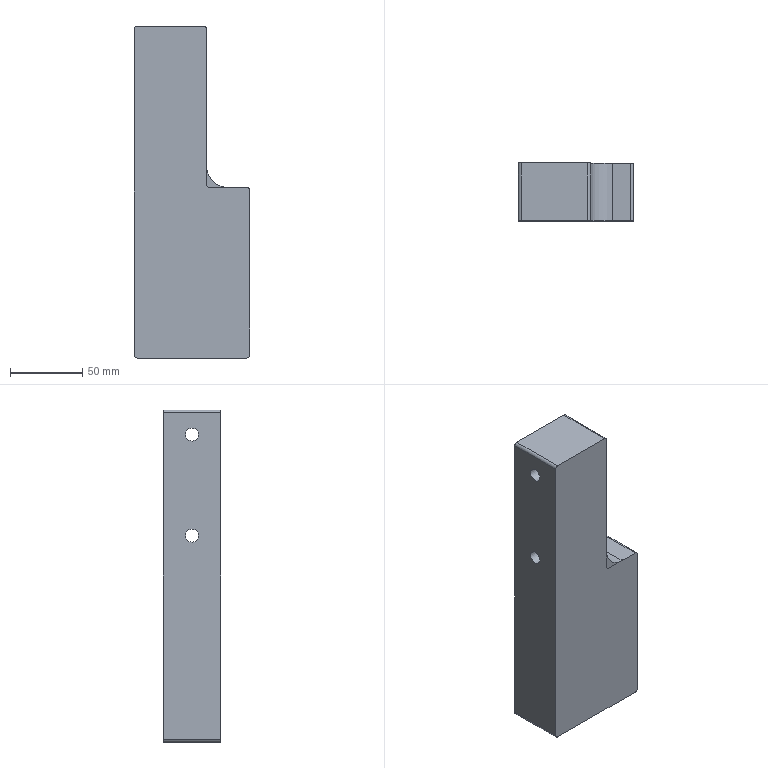NC program | NX | posted with a generic post | part box 80 x 40 x 230 mm
Lines 11495 to 11595 of 15398:
(PLANAR_MILL_COPY_COPY_1_COPY , TOOL : D16.)
N22970 T02 M6
N22972 G53
N22974 G17 G0 G90 X3.093 Y-49.884 B0. C0. S1300 M3
N22976 G43 Z50. H2
N22978 Z-40.15
N22980 G94 G3 X1.1 Y-48.05 R2. F500.
N22982 G1 X-113.
N22984 G2 X-123.05 Y-38. R10.05
N22986 G1 Y38.
N22988 G2 X-113. Y48.05 R10.05
N22990 G1 X113.
N22992 G2 X123.05 Y38. R10.05
N22994 G1 Y-8.1
N22996 G2 X113. Y-18.15 R10.05
N22998 G1 X18.1
N23000 G3 X11.15 Y-25.1 R6.95
N23002 G1 Y-38.
N23004 G2 X1.1 Y-48.05 R10.05
N23006 G3 X-0.9 Y-50.05 R2.
N23008 G0 Z50.
(PLANAR_MILL_COPY_COPY_1_COPY_COPY , TOOL : D16.)
N23010 X3.093 Y-49.833 S800
N23012 Z-40.15
N23014 G3 X1.1 Y-48. R2. F400.
N23016 G1 X-113.
N23018 G2 X-123. Y-38. R10.
N23020 G1 Y38.
N23022 G2 X-113. Y48. R10.
N23024 G1 X113.
N23026 G2 X123. Y38. R10.
N23028 G1 Y-8.1
N23030 G2 X113. Y-18.1 R10.
N23032 G1 X18.1
N23034 G3 X11.1 Y-25.1 R7.
N23036 G1 Y-38.
N23038 G2 X1.1 Y-48. R10.
N23040 G3 X-0.9 Y-50. R2.
N23042 G1 X3.093 Y-49.833
N23044 G3 X1.1 Y-48. R2.
N23046 G1 X-113.
N23048 G2 X-123. Y-38. R10.
N23050 G1 Y38.
N23052 G2 X-113. Y48. R10.
N23054 G1 X113.
N23056 G2 X123. Y38. R10.
N23058 G1 Y-8.1
N23060 G2 X113. Y-18.1 R10.
N23062 G1 X18.1
N23064 G3 X11.1 Y-25.1 R7.
N23066 G1 Y-38.
N23068 G2 X1.1 Y-48. R10.
N23070 G3 X-0.9 Y-50. R2.
N23072 G0 Z50.
N23074 M5
(FLOOR_FACING_COPY_2_1_COPY , TOOL : D63精)
N23076 T20 M6
N23078 G53
N23080 G17 G0 G90 X-156.5 Y24.25 B0. C0. S1600 M3
N23082 G43 Z50. H20
N23084 Z3.
N23086 G94 G1 Z0. F400.
N23088 X-146.5
N23090 X146.5
N23092 Y-8.1
N23094 G2 X145.823 Y-14.8 R33.5
N23096 G1 X-146.5
N23098 X-156.5
N23100 Z3.
N23102 G0 Z50.
N23104 M5
(PLANAR_MILL_COPY_COPY_1 , TOOL : 4倒角)
N23106 T19 M6
N23108 G53
N23110 G17 G0 G90 X-114.967 Y43.136 B0. C0. S4500 M3
N23112 G43 Z50. H19
N23114 Z-1.5
N23116 G94 G3 X-113. Y41.5 R2. F800.
N23118 G1 X113.
N23120 G2 X116.5 Y38. R3.5
N23122 G1 Y-8.1
N23124 G2 X113. Y-11.6 R3.5
N23126 G1 X18.1
N23128 G3 X4.6 Y-25.1 R13.5
N23130 G1 Y-38.
N23132 G2 X1.1 Y-41.5 R3.5
N23134 G1 X-113.
N23136 G2 X-116.5 Y-38. R3.5
N23138 G1 Y38.
N23140 G2 X-113. Y41.5 R3.5
N23142 G3 X-111. Y43.5 R2.
N23144 G0 Z50.
N23146 M5